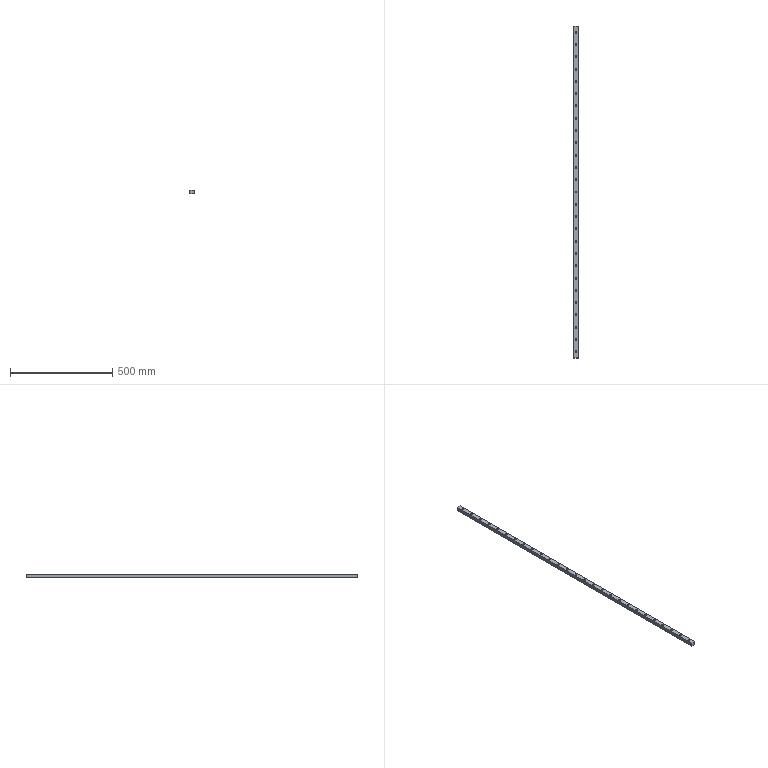Part | STEP file | P-0082097 modified_default | 1 solid | 141 faces | box 20 x 1620 x 18 mm | volume 560839 mm3 | cylinder 108 | plane 33 | commonest cylinder face diameters 5.5 x54 9.5 x54